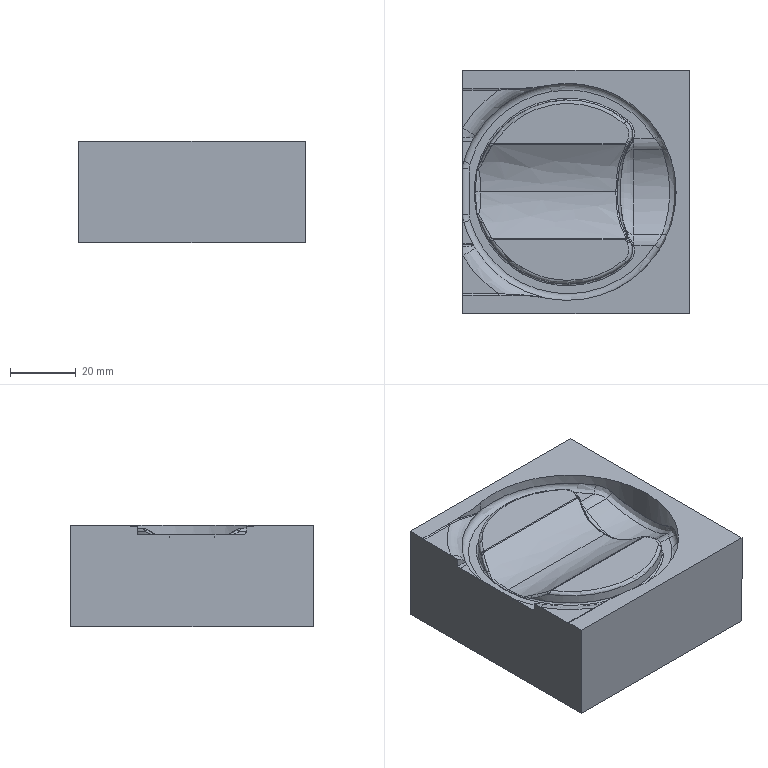CAM job | NX | 3-axis milling | part box 69 x 74 x 31.001 mm | stock box 69 x 74 x 31.005 mm
Tools:
number,name,description,diameter,corner_radius,flute_length,length,flutes
0,D10,Milling Tool-5 Parameters,10.0,0.0,50.0,75.0,2
0,D4,Milling Tool-5 Parameters,4.0,0.0,50.0,75.0,2
0,D3R0.5,Milling Tool-5 Parameters,3.0,0.5,50.0,75.0,2
Operations:
program,operation,operation_type,tool,method,geometry_group,spindle_rpm,surface_speed,feed_per_tooth,feed_cut,feed_plunge,cut_length_mm,path_length_mm,cut_time_min,machine_time_min
NC_PROGRAM,CAVITY_MILL,CavityMilling,D10,METHOD,WORKPIECE,3000.0,282.0,0.4167,2500.0,100.0,7646.724,8031.309,3.059,3.097
NC_PROGRAM,FACE_MILLING,FaceMilling,D10,METHOD,WORKPIECE,3000.0,282.0,0.4167,2500.0,100.0,403.248,455.737,0.1613,0.1665
NC_PROGRAM,CAVITY_MILL_COPY,CavityMilling,D4,METHOD,WORKPIECE,3000.0,282.0,0.4167,2500.0,100.0,10142.337,12302.574,4.057,4.273
NC_PROGRAM,ZLEVEL_PROFILE_COPY,ZLevelMilling,D3R0.5,METHOD,WORKPIECE,3000.0,282.0,0.4167,2500.0,100.0,23912.531,27514.594,9.565,9.925
NC_PROGRAM,FLOOR_WALL,VolumeBased25DMillingOperation,D3R0.5,METHOD,WORKPIECE,3000.0,282.0,0.4167,2500.0,100.0,221.45,357.981,0.0886,0.1022
NC_PROGRAM,CONTOUR_AREA,SurfaceContour,D3R0.5,METHOD,WORKPIECE,3000.0,282.0,0.4167,2500.0,100.0,7743.949,7849.771,3.098,3.108
NC_PROGRAM,CONTOUR_AREA_COPY_COPY,SurfaceContour,D3R0.5,METHOD,MCS_MILL,3000.0,282.0,0.4167,2500.0,100.0,14034.817,14102.852,5.614,5.621